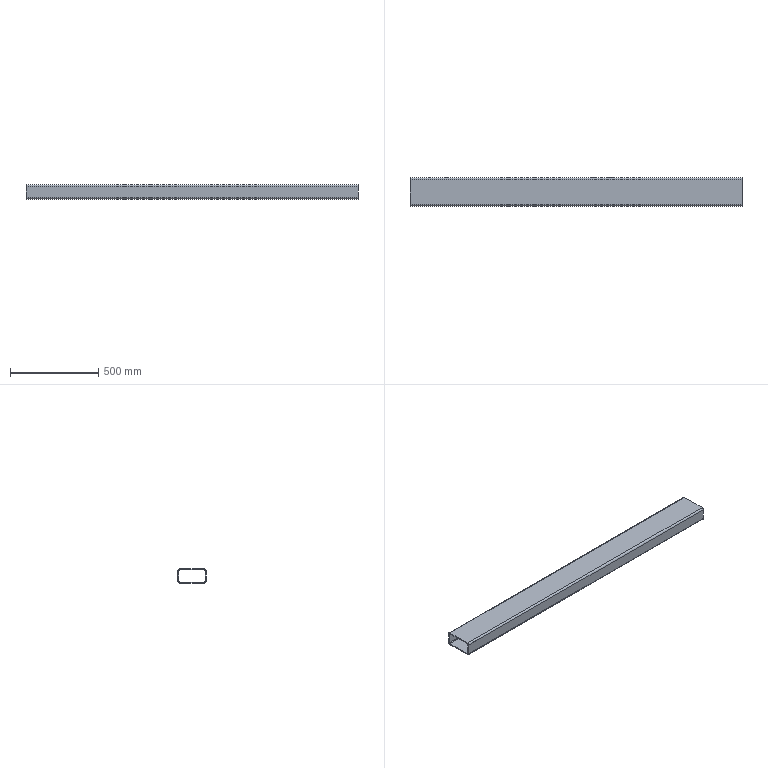Part | SolidWorks | features BaseBody 1 | 1 solid | 26 faces | box 1880 x 160 x 80 mm | volume 4199886 mm3 | cylinder 16 | plane 10 | commonest cylinder face diameters 14 x8 10 x4 20 x4
STEP:
#1=CARTESIAN_POINT('',(-837.,75.,-10.));
#2=VERTEX_POINT('',#1);
#3=CARTESIAN_POINT('',(-823.,75.,-10.));
#4=VERTEX_POINT('',#3);
#5=CARTESIAN_POINT('',(-830.,75.,-10.));
#6=DIRECTION('',(0.,-1.,0.));
#7=DIRECTION('',(0.,0.,-1.));
#8=AXIS2_PLACEMENT_3D('',#5,#6,#7);
#9=CIRCLE('',#8,7.);
#10=EDGE_CURVE('',#2,#4,#9,.T.);
#11=ORIENTED_EDGE('',*,*,#10,.T.);
#12=CARTESIAN_POINT('',(-823.,80.,-10.));
#13=VERTEX_POINT('',#12);
#14=CARTESIAN_POINT('',(-823.,100.,-10.));
#15=DIRECTION('',(0.,1.,0.));
#16=VECTOR('',#15,1000.);
#17=LINE('',#14,#16);
#18=EDGE_CURVE('',#4,#13,#17,.T.);
#19=ORIENTED_EDGE('',*,*,#18,.T.);
#20=CARTESIAN_POINT('',(-837.,80.,-10.));
#21=VERTEX_POINT('',#20);
#22=CARTESIAN_POINT('',(-830.,80.,-10.));
#23=DIRECTION('',(0.,-1.,0.));
#24=DIRECTION('',(0.,0.,-1.));
#25=AXIS2_PLACEMENT_3D('',#22,#23,#24);
#26=CIRCLE('',#25,7.);
#27=EDGE_CURVE('',#21,#13,#26,.T.);
#28=ORIENTED_EDGE('',*,*,#27,.F.);
#29=CARTESIAN_POINT('',(-837.,100.,-10.));
#30=DIRECTION('',(0.,1.,0.));
#31=VECTOR('',#30,1000.);
#32=LINE('',#29,#31);
#33=EDGE_CURVE('',#2,#21,#32,.T.);
#34=ORIENTED_EDGE('',*,*,#33,.F.);
#35=EDGE_LOOP('',(#11,#19,#28,#34));
#36=FACE_OUTER_BOUND('',#35,.T.);
#37=CARTESIAN_POINT('',(-830.,100.,-10.));
#38=DIRECTION('',(0.,1.,0.));
#39=DIRECTION('',(-1.,0.,0.));
#40=AXIS2_PLACEMENT_3D('',#37,#38,#39);
#41=CYLINDRICAL_SURFACE('',#40,7.);
#42=ADVANCED_FACE('',(#36),#41,.F.);
#43=CARTESIAN_POINT('',(-737.,75.,-10.));
#44=VERTEX_POINT('',#43);
#45=CARTESIAN_POINT('',(-723.,75.,-10.));
#46=VERTEX_POINT('',#45);
#47=CARTESIAN_POINT('',(-730.,75.,-10.));
#48=DIRECTION('',(0.,-1.,0.));
#49=DIRECTION('',(0.,0.,-1.));
#50=AXIS2_PLACEMENT_3D('',#47,#48,#49);
#51=CIRCLE('',#50,7.);
#52=EDGE_CURVE('',#44,#46,#51,.T.);
#53=ORIENTED_EDGE('',*,*,#52,.T.);
#54=CARTESIAN_POINT('',(-723.,80.,-10.));
#55=VERTEX_POINT('',#54);
#56=CARTESIAN_POINT('',(-723.,100.,-10.));
#57=DIRECTION('',(0.,1.,0.));
#58=VECTOR('',#57,1000.);
#59=LINE('',#56,#58);
#60=EDGE_CURVE('',#46,#55,#59,.T.);
#61=ORIENTED_EDGE('',*,*,#60,.T.);
#62=CARTESIAN_POINT('',(-737.,80.,-10.));
#63=VERTEX_POINT('',#62);
#64=CARTESIAN_POINT('',(-730.,80.,-10.));
#65=DIRECTION('',(0.,-1.,0.));
#66=DIRECTION('',(0.,0.,-1.));
#67=AXIS2_PLACEMENT_3D('',#64,#65,#66);
#68=CIRCLE('',#67,7.);
#69=EDGE_CURVE('',#63,#55,#68,.T.);
#70=ORIENTED_EDGE('',*,*,#69,.F.);
#71=CARTESIAN_POINT('',(-737.,100.,-10.));
#72=DIRECTION('',(0.,1.,0.));
#73=VECTOR('',#72,1000.);
#74=LINE('',#71,#73);
#75=EDGE_CURVE('',#44,#63,#74,.T.);
#76=ORIENTED_EDGE('',*,*,#75,.F.);
#77=EDGE_LOOP('',(#53,#61,#70,#76));
#78=FACE_OUTER_BOUND('',#77,.T.);
#79=CARTESIAN_POINT('',(-730.,100.,-10.));
#80=DIRECTION('',(0.,1.,0.));
#81=DIRECTION('',(-1.,0.,0.));
#82=AXIS2_PLACEMENT_3D('',#79,#80,#81);
#83=CYLINDRICAL_SURFACE('',#82,7.);
#84=ADVANCED_FACE('',(#78),#83,.F.);
#85=CARTESIAN_POINT('',(88.,75.,-10.));
#86=VERTEX_POINT('',#85);
#87=CARTESIAN_POINT('',(102.,75.,-10.));
#88=VERTEX_POINT('',#87);
#89=CARTESIAN_POINT('',(95.,75.,-10.));
#90=DIRECTION('',(0.,-1.,0.));
#91=DIRECTION('',(0.,0.,-1.));
#92=AXIS2_PLACEMENT_3D('',#89,#90,#91);
#93=CIRCLE('',#92,7.);
#94=EDGE_CURVE('',#86,#88,#93,.T.);
#95=ORIENTED_EDGE('',*,*,#94,.T.);
#96=CARTESIAN_POINT('',(102.,80.,-10.));
#97=VERTEX_POINT('',#96);
#98=CARTESIAN_POINT('',(102.,100.,-10.));
#99=DIRECTION('',(0.,1.,0.));
#100=VECTOR('',#99,1000.);
#101=LINE('',#98,#100);
#102=EDGE_CURVE('',#88,#97,#101,.T.);
#103=ORIENTED_EDGE('',*,*,#102,.T.);
#104=CARTESIAN_POINT('',(88.,80.,-10.));
#105=VERTEX_POINT('',#104);
#106=CARTESIAN_POINT('',(95.,80.,-10.));
#107=DIRECTION('',(0.,-1.,0.));
#108=DIRECTION('',(0.,0.,-1.));
#109=AXIS2_PLACEMENT_3D('',#106,#107,#108);
#110=CIRCLE('',#109,7.);
#111=EDGE_CURVE('',#105,#97,#110,.T.);
#112=ORIENTED_EDGE('',*,*,#111,.F.);
#113=CARTESIAN_POINT('',(88.,100.,-10.));
#114=DIRECTION('',(0.,1.,0.));
#115=VECTOR('',#114,1000.);
#116=LINE('',#113,#115);
#117=EDGE_CURVE('',#86,#105,#116,.T.);
#118=ORIENTED_EDGE('',*,*,#117,.F.);
#119=EDGE_LOOP('',(#95,#103,#112,#118));
#120=FACE_OUTER_BOUND('',#119,.T.);
#121=CARTESIAN_POINT('',(95.,100.,-10.));
#122=DIRECTION('',(0.,1.,0.));
#123=DIRECTION('',(-1.,0.,0.));
#124=AXIS2_PLACEMENT_3D('',#121,#122,#123);
#125=CYLINDRICAL_SURFACE('',#124,7.);
#126=ADVANCED_FACE('',(#120),#125,.F.);
#127=CARTESIAN_POINT('',(188.,75.,-10.));
#128=VERTEX_POINT('',#127);
#129=CARTESIAN_POINT('',(202.,75.,-10.));
#130=VERTEX_POINT('',#129);
#131=CARTESIAN_POINT('',(195.,75.,-10.));
#132=DIRECTION('',(0.,-1.,0.));
#133=DIRECTION('',(0.,0.,-1.));
#134=AXIS2_PLACEMENT_3D('',#131,#132,#133);
#135=CIRCLE('',#134,7.);
#136=EDGE_CURVE('',#128,#130,#135,.T.);
#137=ORIENTED_EDGE('',*,*,#136,.T.);
#138=CARTESIAN_POINT('',(202.,80.,-10.));
#139=VERTEX_POINT('',#138);
#140=CARTESIAN_POINT('',(202.,100.,-10.));
#141=DIRECTION('',(0.,1.,0.));
#142=VECTOR('',#141,1000.);
#143=LINE('',#140,#142);
#144=EDGE_CURVE('',#130,#139,#143,.T.);
#145=ORIENTED_EDGE('',*,*,#144,.T.);
#146=CARTESIAN_POINT('',(188.,80.,-10.));
#147=VERTEX_POINT('',#146);
#148=CARTESIAN_POINT('',(195.,80.,-10.));
#149=DIRECTION('',(0.,-1.,0.));
#150=DIRECTION('',(0.,0.,-1.));
#151=AXIS2_PLACEMENT_3D('',#148,#149,#150);
#152=CIRCLE('',#151,7.);
#153=EDGE_CURVE('',#147,#139,#152,.T.);
#154=ORIENTED_EDGE('',*,*,#153,.F.);
#155=CARTESIAN_POINT('',(188.,100.,-10.));
#156=DIRECTION('',(0.,1.,0.));
#157=VECTOR('',#156,1000.);
#158=LINE('',#155,#157);
#159=EDGE_CURVE('',#128,#147,#158,.T.);
#160=ORIENTED_EDGE('',*,*,#159,.F.);
#161=EDGE_LOOP('',(#137,#145,#154,#160));
#162=FACE_OUTER_BOUND('',#161,.T.);
#163=CARTESIAN_POINT('',(195.,100.,-10.));
#164=DIRECTION('',(0.,1.,0.));
#165=DIRECTION('',(-1.,0.,0.));
#166=AXIS2_PLACEMENT_3D('',#163,#164,#165);
#167=CYLINDRICAL_SURFACE('',#166,7.);
#168=ADVANCED_FACE('',(#162),#167,.F.);
#169=CARTESIAN_POINT('',(-940.,70.,-40.));
#170=VERTEX_POINT('',#169);
#171=CARTESIAN_POINT('',(-940.,80.,-30.));
#172=VERTEX_POINT('',#171);
#173=CARTESIAN_POINT('',(-940.,70.,-30.));
#174=DIRECTION('',(1.,0.,0.));
#175=DIRECTION('',(0.,0.,-1.));
#176=AXIS2_PLACEMENT_3D('',#173,#174,#175);
#177=CIRCLE('',#176,10.);
#178=EDGE_CURVE('',#170,#172,#177,.T.);
#179=ORIENTED_EDGE('',*,*,#178,.T.);
#180=CARTESIAN_POINT('',(940.,80.,-30.));
#181=VERTEX_POINT('',#180);
#182=CARTESIAN_POINT('',(940.,80.,-30.));
#183=DIRECTION('',(-1.,0.,0.));
#184=VECTOR('',#183,1000.);
#185=LINE('',#182,#184);
#186=EDGE_CURVE('',#181,#172,#185,.T.);
#187=ORIENTED_EDGE('',*,*,#186,.F.);
#188=CARTESIAN_POINT('',(940.,70.,-40.));
#189=VERTEX_POINT('',#188);
#190=CARTESIAN_POINT('',(940.,70.,-30.));
#191=DIRECTION('',(1.,0.,0.));
#192=DIRECTION('',(0.,0.,-1.));
#193=AXIS2_PLACEMENT_3D('',#190,#191,#192);
#194=CIRCLE('',#193,10.);
#195=EDGE_CURVE('',#189,#181,#194,.T.);
#196=ORIENTED_EDGE('',*,*,#195,.F.);
#197=CARTESIAN_POINT('',(940.,70.,-40.));
#198=DIRECTION('',(-1.,0.,0.));
#199=VECTOR('',#198,1000.);
#200=LINE('',#197,#199);
#201=EDGE_CURVE('',#189,#170,#200,.T.);
#202=ORIENTED_EDGE('',*,*,#201,.T.);
#203=EDGE_LOOP('',(#179,#187,#196,#202));
#204=FACE_OUTER_BOUND('',#203,.T.);
#205=CARTESIAN_POINT('',(940.,70.,-30.));
#206=DIRECTION('',(-1.,0.,0.));
#207=DIRECTION('',(0.,0.,1.));
#208=AXIS2_PLACEMENT_3D('',#205,#206,#207);
#209=CYLINDRICAL_SURFACE('',#208,10.);
#210=ADVANCED_FACE('',(#204),#209,.T.);
#211=ORIENTED_EDGE('',*,*,#27,.T.);
#212=CARTESIAN_POINT('',(-830.,80.,-10.));
#213=DIRECTION('',(0.,-1.,0.));
#214=DIRECTION('',(0.,0.,-1.));
#215=AXIS2_PLACEMENT_3D('',#212,#213,#214);
#216=CIRCLE('',#215,7.);
#217=EDGE_CURVE('',#13,#21,#216,.T.);
#218=ORIENTED_EDGE('',*,*,#217,.T.);
#219=EDGE_LOOP('',(#211,#218));
#220=FACE_BOUND('',#219,.T.);
#221=ORIENTED_EDGE('',*,*,#69,.T.);
#222=CARTESIAN_POINT('',(-730.,80.,-10.));
#223=DIRECTION('',(0.,-1.,0.));
#224=DIRECTION('',(0.,0.,-1.));
#225=AXIS2_PLACEMENT_3D('',#222,#223,#224);
#226=CIRCLE('',#225,7.);
#227=EDGE_CURVE('',#55,#63,#226,.T.);
#228=ORIENTED_EDGE('',*,*,#227,.T.);
#229=EDGE_LOOP('',(#221,#228));
#230=FACE_BOUND('',#229,.T.);
#231=ORIENTED_EDGE('',*,*,#111,.T.);
#232=CARTESIAN_POINT('',(95.,80.,-10.));
#233=DIRECTION('',(0.,-1.,0.));
#234=DIRECTION('',(0.,0.,-1.));
#235=AXIS2_PLACEMENT_3D('',#232,#233,#234);
#236=CIRCLE('',#235,7.);
#237=EDGE_CURVE('',#97,#105,#236,.T.);
#238=ORIENTED_EDGE('',*,*,#237,.T.);
#239=EDGE_LOOP('',(#231,#238));
#240=FACE_BOUND('',#239,.T.);
#241=ORIENTED_EDGE('',*,*,#153,.T.);
#242=CARTESIAN_POINT('',(195.,80.,-10.));
#243=DIRECTION('',(0.,-1.,0.));
#244=DIRECTION('',(0.,0.,-1.));
#245=AXIS2_PLACEMENT_3D('',#242,#243,#244);
#246=CIRCLE('',#245,7.);
#247=EDGE_CURVE('',#139,#147,#246,.T.);
#248=ORIENTED_EDGE('',*,*,#247,.T.);
#249=EDGE_LOOP('',(#241,#248));
#250=FACE_BOUND('',#249,.T.);
#251=CARTESIAN_POINT('',(-940.,80.,30.));
#252=VERTEX_POINT('',#251);
#253=CARTESIAN_POINT('',(-940.,80.,-30.));
#254=DIRECTION('',(0.,0.,1.));
#255=VECTOR('',#254,1000.);
#256=LINE('',#253,#255);
#257=EDGE_CURVE('',#172,#252,#256,.T.);
#258=ORIENTED_EDGE('',*,*,#257,.T.);
#259=CARTESIAN_POINT('',(940.,80.,30.));
#260=VERTEX_POINT('',#259);
#261=CARTESIAN_POINT('',(940.,80.,30.));
#262=DIRECTION('',(-1.,0.,0.));
#263=VECTOR('',#262,1000.);
#264=LINE('',#261,#263);
#265=EDGE_CURVE('',#260,#252,#264,.T.);
#266=ORIENTED_EDGE('',*,*,#265,.F.);
#267=CARTESIAN_POINT('',(940.,80.,-30.));
#268=DIRECTION('',(0.,0.,1.));
#269=VECTOR('',#268,1000.);
#270=LINE('',#267,#269);
#271=EDGE_CURVE('',#181,#260,#270,.T.);
#272=ORIENTED_EDGE('',*,*,#271,.F.);
#273=ORIENTED_EDGE('',*,*,#186,.T.);
#274=EDGE_LOOP('',(#258,#266,#272,#273));
#275=FACE_OUTER_BOUND('',#274,.T.);
#276=CARTESIAN_POINT('',(940.,80.,-30.));
#277=DIRECTION('',(0.,-1.,0.));
#278=DIRECTION('',(0.,0.,-1.));
#279=AXIS2_PLACEMENT_3D('',#276,#277,#278);
#280=PLANE('',#279);
#281=ADVANCED_FACE('',(#220,#230,#240,#250,#275),#280,.F.);
#282=CARTESIAN_POINT('',(-940.,70.,40.));
#283=VERTEX_POINT('',#282);
#284=CARTESIAN_POINT('',(-940.,70.,30.));
#285=DIRECTION('',(1.,0.,0.));
#286=DIRECTION('',(0.,0.,-1.));
#287=AXIS2_PLACEMENT_3D('',#284,#285,#286);
#288=CIRCLE('',#287,10.);
#289=EDGE_CURVE('',#252,#283,#288,.T.);
#290=ORIENTED_EDGE('',*,*,#289,.T.);
#291=CARTESIAN_POINT('',(940.,70.,40.));
#292=VERTEX_POINT('',#291);
#293=CARTESIAN_POINT('',(940.,70.,40.));
#294=DIRECTION('',(-1.,0.,0.));
#295=VECTOR('',#294,1000.);
#296=LINE('',#293,#295);
#297=EDGE_CURVE('',#292,#283,#296,.T.);
#298=ORIENTED_EDGE('',*,*,#297,.F.);
#299=CARTESIAN_POINT('',(940.,70.,30.));
#300=DIRECTION('',(1.,0.,0.));
#301=DIRECTION('',(0.,0.,-1.));
#302=AXIS2_PLACEMENT_3D('',#299,#300,#301);
#303=CIRCLE('',#302,10.);
#304=EDGE_CURVE('',#260,#292,#303,.T.);
#305=ORIENTED_EDGE('',*,*,#304,.F.);
#306=ORIENTED_EDGE('',*,*,#265,.T.);
#307=EDGE_LOOP('',(#290,#298,#305,#306));
#308=FACE_OUTER_BOUND('',#307,.T.);
#309=CARTESIAN_POINT('',(940.,70.,30.));
#310=DIRECTION('',(-1.,0.,0.));
#311=DIRECTION('',(0.,0.,1.));
#312=AXIS2_PLACEMENT_3D('',#309,#310,#311);
#313=CYLINDRICAL_SURFACE('',#312,10.);
#314=ADVANCED_FACE('',(#308),#313,.T.);
#315=CARTESIAN_POINT('',(-940.,-70.,40.));
#316=VERTEX_POINT('',#315);
#317=CARTESIAN_POINT('',(-940.,-70.,40.));
#318=DIRECTION('',(0.,-1.,0.));
#319=VECTOR('',#318,1000.);
#320=LINE('',#317,#319);
#321=EDGE_CURVE('',#283,#316,#320,.T.);
#322=ORIENTED_EDGE('',*,*,#321,.T.);
#323=CARTESIAN_POINT('',(940.,-70.,40.));
#324=VERTEX_POINT('',#323);
#325=CARTESIAN_POINT('',(940.,-70.,40.));
#326=DIRECTION('',(-1.,0.,0.));
#327=VECTOR('',#326,1000.);
#328=LINE('',#325,#327);
#329=EDGE_CURVE('',#324,#316,#328,.T.);
#330=ORIENTED_EDGE('',*,*,#329,.F.);
#331=CARTESIAN_POINT('',(940.,-70.,40.));
#332=DIRECTION('',(0.,-1.,0.));
#333=VECTOR('',#332,1000.);
#334=LINE('',#331,#333);
#335=EDGE_CURVE('',#292,#324,#334,.T.);
#336=ORIENTED_EDGE('',*,*,#335,.F.);
#337=ORIENTED_EDGE('',*,*,#297,.T.);
#338=EDGE_LOOP('',(#322,#330,#336,#337));
#339=FACE_OUTER_BOUND('',#338,.T.);
#340=CARTESIAN_POINT('',(940.,-70.,40.));
#341=DIRECTION('',(0.,0.,-1.));
#342=DIRECTION('',(0.,1.,0.));
#343=AXIS2_PLACEMENT_3D('',#340,#341,#342);
#344=PLANE('',#343);
#345=ADVANCED_FACE('',(#339),#344,.F.);
#346=CARTESIAN_POINT('',(-940.,-80.,30.));
#347=VERTEX_POINT('',#346);
#348=CARTESIAN_POINT('',(-940.,-70.,30.));
#349=DIRECTION('',(1.,0.,0.));
#350=DIRECTION('',(0.,0.,-1.));
#351=AXIS2_PLACEMENT_3D('',#348,#349,#350);
#352=CIRCLE('',#351,10.);
#353=EDGE_CURVE('',#316,#347,#352,.T.);
#354=ORIENTED_EDGE('',*,*,#353,.T.);
#355=CARTESIAN_POINT('',(940.,-80.,30.));
#356=VERTEX_POINT('',#355);
#357=CARTESIAN_POINT('',(940.,-80.,30.));
#358=DIRECTION('',(-1.,0.,0.));
#359=VECTOR('',#358,1000.);
#360=LINE('',#357,#359);
#361=EDGE_CURVE('',#356,#347,#360,.T.);
#362=ORIENTED_EDGE('',*,*,#361,.F.);
#363=CARTESIAN_POINT('',(940.,-70.,30.));
#364=DIRECTION('',(1.,0.,0.));
#365=DIRECTION('',(0.,0.,-1.));
#366=AXIS2_PLACEMENT_3D('',#363,#364,#365);
#367=CIRCLE('',#366,10.);
#368=EDGE_CURVE('',#324,#356,#367,.T.);
#369=ORIENTED_EDGE('',*,*,#368,.F.);
#370=ORIENTED_EDGE('',*,*,#329,.T.);
#371=EDGE_LOOP('',(#354,#362,#369,#370));
#372=FACE_OUTER_BOUND('',#371,.T.);
#373=CARTESIAN_POINT('',(940.,-70.,30.));
#374=DIRECTION('',(-1.,0.,0.));
#375=DIRECTION('',(0.,0.,1.));
#376=AXIS2_PLACEMENT_3D('',#373,#374,#375);
#377=CYLINDRICAL_SURFACE('',#376,10.);
#378=ADVANCED_FACE('',(#372),#377,.T.);
#379=CARTESIAN_POINT('',(-940.,-80.,-30.));
#380=VERTEX_POINT('',#379);
#381=CARTESIAN_POINT('',(-940.,-80.,30.));
#382=DIRECTION('',(0.,0.,-1.));
#383=VECTOR('',#382,1000.);
#384=LINE('',#381,#383);
#385=EDGE_CURVE('',#347,#380,#384,.T.);
#386=ORIENTED_EDGE('',*,*,#385,.T.);
#387=CARTESIAN_POINT('',(940.,-80.,-30.));
#388=VERTEX_POINT('',#387);
#389=CARTESIAN_POINT('',(940.,-80.,-30.));
#390=DIRECTION('',(-1.,0.,0.));
#391=VECTOR('',#390,1000.);
#392=LINE('',#389,#391);
#393=EDGE_CURVE('',#388,#380,#392,.T.);
#394=ORIENTED_EDGE('',*,*,#393,.F.);
#395=CARTESIAN_POINT('',(940.,-80.,30.));
#396=DIRECTION('',(0.,0.,-1.));
#397=VECTOR('',#396,1000.);
#398=LINE('',#395,#397);
#399=EDGE_CURVE('',#356,#388,#398,.T.);
#400=ORIENTED_EDGE('',*,*,#399,.F.);
#401=ORIENTED_EDGE('',*,*,#361,.T.);
#402=EDGE_LOOP('',(#386,#394,#400,#401));
#403=FACE_OUTER_BOUND('',#402,.T.);
#404=CARTESIAN_POINT('',(940.,-80.,30.));
#405=DIRECTION('',(0.,1.,0.));
#406=DIRECTION('',(0.,0.,1.));
#407=AXIS2_PLACEMENT_3D('',#404,#405,#406);
#408=PLANE('',#407);
#409=ADVANCED_FACE('',(#403),#408,.F.);
#410=CARTESIAN_POINT('',(-940.,-70.,-40.));
#411=VERTEX_POINT('',#410);
#412=CARTESIAN_POINT('',(-940.,-70.,-30.));
#413=DIRECTION('',(1.,0.,0.));
#414=DIRECTION('',(0.,0.,-1.));
#415=AXIS2_PLACEMENT_3D('',#412,#413,#414);
#416=CIRCLE('',#415,10.);
#417=EDGE_CURVE('',#380,#411,#416,.T.);
#418=ORIENTED_EDGE('',*,*,#417,.T.);
#419=CARTESIAN_POINT('',(940.,-70.,-40.));
#420=VERTEX_POINT('',#419);
#421=CARTESIAN_POINT('',(940.,-70.,-40.));
#422=DIRECTION('',(-1.,0.,0.));
#423=VECTOR('',#422,1000.);
#424=LINE('',#421,#423);
#425=EDGE_CURVE('',#420,#411,#424,.T.);
#426=ORIENTED_EDGE('',*,*,#425,.F.);
#427=CARTESIAN_POINT('',(940.,-70.,-30.));
#428=DIRECTION('',(1.,0.,0.));
#429=DIRECTION('',(0.,0.,-1.));
#430=AXIS2_PLACEMENT_3D('',#427,#428,#429);
#431=CIRCLE('',#430,10.);
#432=EDGE_CURVE('',#388,#420,#431,.T.);
#433=ORIENTED_EDGE('',*,*,#432,.F.);
#434=ORIENTED_EDGE('',*,*,#393,.T.);
#435=EDGE_LOOP('',(#418,#426,#433,#434));
#436=FACE_OUTER_BOUND('',#435,.T.);
#437=CARTESIAN_POINT('',(940.,-70.,-30.));
#438=DIRECTION('',(-1.,0.,0.));
#439=DIRECTION('',(0.,0.,1.));
#440=AXIS2_PLACEMENT_3D('',#437,#438,#439);
#441=CYLINDRICAL_SURFACE('',#440,10.);
#442=ADVANCED_FACE('',(#436),#441,.T.);
#443=CARTESIAN_POINT('',(-940.,75.,30.));
#444=VERTEX_POINT('',#443);
#445=CARTESIAN_POINT('',(-940.,70.,35.));
#446=VERTEX_POINT('',#445);
#447=CARTESIAN_POINT('',(-940.,70.,30.));
#448=DIRECTION('',(1.,0.,0.));
#449=DIRECTION('',(0.,0.,-1.));
#450=AXIS2_PLACEMENT_3D('',#447,#448,#449);
#451=CIRCLE('',#450,5.);
#452=EDGE_CURVE('',#444,#446,#451,.T.);
#453=ORIENTED_EDGE('',*,*,#452,.F.);
#454=CARTESIAN_POINT('',(940.,75.,30.));
#455=VERTEX_POINT('',#454);
#456=CARTESIAN_POINT('',(940.,75.,30.));
#457=DIRECTION('',(-1.,0.,0.));
#458=VECTOR('',#457,1000.);
#459=LINE('',#456,#458);
#460=EDGE_CURVE('',#455,#444,#459,.T.);
#461=ORIENTED_EDGE('',*,*,#460,.F.);
#462=CARTESIAN_POINT('',(940.,70.,35.));
#463=VERTEX_POINT('',#462);
#464=CARTESIAN_POINT('',(940.,70.,30.));
#465=DIRECTION('',(1.,0.,0.));
#466=DIRECTION('',(0.,0.,-1.));
#467=AXIS2_PLACEMENT_3D('',#464,#465,#466);
#468=CIRCLE('',#467,5.);
#469=EDGE_CURVE('',#455,#463,#468,.T.);
#470=ORIENTED_EDGE('',*,*,#469,.T.);
#471=CARTESIAN_POINT('',(940.,70.,35.));
#472=DIRECTION('',(-1.,0.,0.));
#473=VECTOR('',#472,1000.);
#474=LINE('',#471,#473);
#475=EDGE_CURVE('',#463,#446,#474,.T.);
#476=ORIENTED_EDGE('',*,*,#475,.T.);
#477=EDGE_LOOP('',(#453,#461,#470,#476));
#478=FACE_OUTER_BOUND('',#477,.T.);
#479=CARTESIAN_POINT('',(940.,70.,30.));
#480=DIRECTION('',(-1.,0.,0.));
#481=DIRECTION('',(0.,0.,1.));
#482=AXIS2_PLACEMENT_3D('',#479,#480,#481);
#483=CYLINDRICAL_SURFACE('',#482,5.);
#484=ADVANCED_FACE('',(#478),#483,.F.);
#485=ORIENTED_EDGE('',*,*,#10,.F.);
#486=CARTESIAN_POINT('',(-830.,75.,-10.));
#487=DIRECTION('',(0.,-1.,0.));
#488=DIRECTION('',(0.,0.,-1.));
#489=AXIS2_PLACEMENT_3D('',#486,#487,#488);
#490=CIRCLE('',#489,7.);
#491=EDGE_CURVE('',#4,#2,#490,.T.);
#492=ORIENTED_EDGE('',*,*,#491,.F.);
#493=EDGE_LOOP('',(#485,#492));
#494=FACE_BOUND('',#493,.T.);
#495=ORIENTED_EDGE('',*,*,#52,.F.);
#496=CARTESIAN_POINT('',(-730.,75.,-10.));
#497=DIRECTION('',(0.,-1.,0.));
#498=DIRECTION('',(0.,0.,-1.));
#499=AXIS2_PLACEMENT_3D('',#496,#497,#498);
#500=CIRCLE('',#499,7.);
#501=EDGE_CURVE('',#46,#44,#500,.T.);
#502=ORIENTED_EDGE('',*,*,#501,.F.);
#503=EDGE_LOOP('',(#495,#502));
#504=FACE_BOUND('',#503,.T.);
#505=ORIENTED_EDGE('',*,*,#94,.F.);
#506=CARTESIAN_POINT('',(95.,75.,-10.));
#507=DIRECTION('',(0.,-1.,0.));
#508=DIRECTION('',(0.,0.,-1.));
#509=AXIS2_PLACEMENT_3D('',#506,#507,#508);
#510=CIRCLE('',#509,7.);
#511=EDGE_CURVE('',#88,#86,#510,.T.);
#512=ORIENTED_EDGE('',*,*,#511,.F.);
#513=EDGE_LOOP('',(#505,#512));
#514=FACE_BOUND('',#513,.T.);
#515=ORIENTED_EDGE('',*,*,#136,.F.);
#516=CARTESIAN_POINT('',(195.,75.,-10.));
#517=DIRECTION('',(0.,-1.,0.));
#518=DIRECTION('',(0.,0.,-1.));
#519=AXIS2_PLACEMENT_3D('',#516,#517,#518);
#520=CIRCLE('',#519,7.);
#521=EDGE_CURVE('',#130,#128,#520,.T.);
#522=ORIENTED_EDGE('',*,*,#521,.F.);
#523=EDGE_LOOP('',(#515,#522));
#524=FACE_BOUND('',#523,.T.);
#525=CARTESIAN_POINT('',(-940.,75.,-30.));
#526=VERTEX_POINT('',#525);
#527=CARTESIAN_POINT('',(-940.,75.,-30.));
#528=DIRECTION('',(0.,0.,1.));
#529=VECTOR('',#528,1000.);
#530=LINE('',#527,#529);
#531=EDGE_CURVE('',#526,#444,#530,.T.);
#532=ORIENTED_EDGE('',*,*,#531,.F.);
#533=CARTESIAN_POINT('',(940.,75.,-30.));
#534=VERTEX_POINT('',#533);
#535=CARTESIAN_POINT('',(940.,75.,-30.));
#536=DIRECTION('',(-1.,0.,0.));
#537=VECTOR('',#536,1000.);
#538=LINE('',#535,#537);
#539=EDGE_CURVE('',#534,#526,#538,.T.);
#540=ORIENTED_EDGE('',*,*,#539,.F.);
#541=CARTESIAN_POINT('',(940.,75.,-30.));
#542=DIRECTION('',(0.,0.,1.));
#543=VECTOR('',#542,1000.);
#544=LINE('',#541,#543);
#545=EDGE_CURVE('',#534,#455,#544,.T.);
#546=ORIENTED_EDGE('',*,*,#545,.T.);
#547=ORIENTED_EDGE('',*,*,#460,.T.);
#548=EDGE_LOOP('',(#532,#540,#546,#547));
#549=FACE_OUTER_BOUND('',#548,.T.);
#550=CARTESIAN_POINT('',(940.,75.,-30.));
#551=DIRECTION('',(0.,-1.,0.));
#552=DIRECTION('',(0.,0.,-1.));
#553=AXIS2_PLACEMENT_3D('',#550,#551,#552);
#554=PLANE('',#553);
#555=ADVANCED_FACE('',(#494,#504,#514,#524,#549),#554,.T.);
#556=CARTESIAN_POINT('',(-940.,70.,-35.));
#557=VERTEX_POINT('',#556);
#558=CARTESIAN_POINT('',(-940.,70.,-30.));
#559=DIRECTION('',(1.,0.,0.));
#560=DIRECTION('',(0.,0.,-1.));
#561=AXIS2_PLACEMENT_3D('',#558,#559,#560);
#562=CIRCLE('',#561,5.);
#563=EDGE_CURVE('',#557,#526,#562,.T.);
#564=ORIENTED_EDGE('',*,*,#563,.F.);
#565=CARTESIAN_POINT('',(940.,70.,-35.));
#566=VERTEX_POINT('',#565);
#567=CARTESIAN_POINT('',(940.,70.,-35.));
#568=DIRECTION('',(-1.,0.,0.));
#569=VECTOR('',#568,1000.);
#570=LINE('',#567,#569);
#571=EDGE_CURVE('',#566,#557,#570,.T.);
#572=ORIENTED_EDGE('',*,*,#571,.F.);
#573=CARTESIAN_POINT('',(940.,70.,-30.));
#574=DIRECTION('',(1.,0.,0.));
#575=DIRECTION('',(0.,0.,-1.));
#576=AXIS2_PLACEMENT_3D('',#573,#574,#575);
#577=CIRCLE('',#576,5.);
#578=EDGE_CURVE('',#566,#534,#577,.T.);
#579=ORIENTED_EDGE('',*,*,#578,.T.);
#580=ORIENTED_EDGE('',*,*,#539,.T.);
#581=EDGE_LOOP('',(#564,#572,#579,#580));
#582=FACE_OUTER_BOUND('',#581,.T.);
#583=CARTESIAN_POINT('',(940.,70.,-30.));
#584=DIRECTION('',(-1.,0.,0.));
#585=DIRECTION('',(0.,0.,1.));
#586=AXIS2_PLACEMENT_3D('',#583,#584,#585);
#587=CYLINDRICAL_SURFACE('',#586,5.);
#588=ADVANCED_FACE('',(#582),#587,.F.);
#589=CARTESIAN_POINT('',(-940.,-70.,-35.));
#590=VERTEX_POINT('',#589);
#591=CARTESIAN_POINT('',(-940.,70.,-35.));
#592=DIRECTION('',(0.,1.,0.));
#593=VECTOR('',#592,1000.);
#594=LINE('',#591,#593);
#595=EDGE_CURVE('',#590,#557,#594,.T.);
#596=ORIENTED_EDGE('',*,*,#595,.F.);
#597=CARTESIAN_POINT('',(940.,-70.,-35.));
#598=VERTEX_POINT('',#597);
#599=CARTESIAN_POINT('',(940.,-70.,-35.));
#600=DIRECTION('',(-1.,0.,0.));
#601=VECTOR('',#600,1000.);
#602=LINE('',#599,#601);
#603=EDGE_CURVE('',#598,#590,#602,.T.);
#604=ORIENTED_EDGE('',*,*,#603,.F.);
#605=CARTESIAN_POINT('',(940.,70.,-35.));
#606=DIRECTION('',(0.,1.,0.));
#607=VECTOR('',#606,1000.);
#608=LINE('',#605,#607);
#609=EDGE_CURVE('',#598,#566,#608,.T.);
#610=ORIENTED_EDGE('',*,*,#609,.T.);
#611=ORIENTED_EDGE('',*,*,#571,.T.);
#612=EDGE_LOOP('',(#596,#604,#610,#611));
#613=FACE_OUTER_BOUND('',#612,.T.);
#614=CARTESIAN_POINT('',(940.,70.,-35.));
#615=DIRECTION('',(0.,0.,1.));
#616=DIRECTION('',(1.,0.,0.));
#617=AXIS2_PLACEMENT_3D('',#614,#615,#616);
#618=PLANE('',#617);
#619=ADVANCED_FACE('',(#613),#618,.T.);
#620=CARTESIAN_POINT('',(-940.,-75.,-30.));
#621=VERTEX_POINT('',#620);
#622=CARTESIAN_POINT('',(-940.,-70.,-30.));
#623=DIRECTION('',(1.,0.,0.));
#624=DIRECTION('',(0.,0.,-1.));
#625=AXIS2_PLACEMENT_3D('',#622,#623,#624);
#626=CIRCLE('',#625,5.);
#627=EDGE_CURVE('',#621,#590,#626,.T.);
#628=ORIENTED_EDGE('',*,*,#627,.F.);
#629=CARTESIAN_POINT('',(940.,-75.,-30.));
#630=VERTEX_POINT('',#629);
#631=CARTESIAN_POINT('',(940.,-75.,-30.));
#632=DIRECTION('',(-1.,0.,0.));
#633=VECTOR('',#632,1000.);
#634=LINE('',#631,#633);
#635=EDGE_CURVE('',#630,#621,#634,.T.);
#636=ORIENTED_EDGE('',*,*,#635,.F.);
#637=CARTESIAN_POINT('',(940.,-70.,-30.));
#638=DIRECTION('',(1.,0.,0.));
#639=DIRECTION('',(0.,0.,-1.));
#640=AXIS2_PLACEMENT_3D('',#637,#638,#639);
#641=CIRCLE('',#640,5.);
#642=EDGE_CURVE('',#630,#598,#641,.T.);
#643=ORIENTED_EDGE('',*,*,#642,.T.);
#644=ORIENTED_EDGE('',*,*,#603,.T.);
#645=EDGE_LOOP('',(#628,#636,#643,#644));
#646=FACE_OUTER_BOUND('',#645,.T.);
#647=CARTESIAN_POINT('',(940.,-70.,-30.));
#648=DIRECTION('',(-1.,0.,0.));
#649=DIRECTION('',(0.,0.,1.));
#650=AXIS2_PLACEMENT_3D('',#647,#648,#649);
#651=CYLINDRICAL_SURFACE('',#650,5.);
#652=ADVANCED_FACE('',(#646),#651,.F.);
#653=CARTESIAN_POINT('',(-940.,-75.,30.));
#654=VERTEX_POINT('',#653);
#655=CARTESIAN_POINT('',(-940.,-75.,30.));
#656=DIRECTION('',(0.,0.,-1.));
#657=VECTOR('',#656,1000.);
#658=LINE('',#655,#657);
#659=EDGE_CURVE('',#654,#621,#658,.T.);
#660=ORIENTED_EDGE('',*,*,#659,.F.);
#661=CARTESIAN_POINT('',(940.,-75.,30.));
#662=VERTEX_POINT('',#661);
#663=CARTESIAN_POINT('',(940.,-75.,30.));
#664=DIRECTION('',(-1.,0.,0.));
#665=VECTOR('',#664,1000.);
#666=LINE('',#663,#665);
#667=EDGE_CURVE('',#662,#654,#666,.T.);
#668=ORIENTED_EDGE('',*,*,#667,.F.);
#669=CARTESIAN_POINT('',(940.,-75.,30.));
#670=DIRECTION('',(0.,0.,-1.));
#671=VECTOR('',#670,1000.);
#672=LINE('',#669,#671);
#673=EDGE_CURVE('',#662,#630,#672,.T.);
#674=ORIENTED_EDGE('',*,*,#673,.T.);
#675=ORIENTED_EDGE('',*,*,#635,.T.);
#676=EDGE_LOOP('',(#660,#668,#674,#675));
#677=FACE_OUTER_BOUND('',#676,.T.);
#678=CARTESIAN_POINT('',(940.,-75.,30.));
#679=DIRECTION('',(0.,1.,0.));
#680=DIRECTION('',(0.,0.,1.));
#681=AXIS2_PLACEMENT_3D('',#678,#679,#680);
#682=PLANE('',#681);
#683=ADVANCED_FACE('',(#677),#682,.T.);
#684=CARTESIAN_POINT('',(-940.,-70.,35.));
#685=VERTEX_POINT('',#684);
#686=CARTESIAN_POINT('',(-940.,-70.,30.));
#687=DIRECTION('',(1.,0.,0.));
#688=DIRECTION('',(0.,0.,-1.));
#689=AXIS2_PLACEMENT_3D('',#686,#687,#688);
#690=CIRCLE('',#689,5.);
#691=EDGE_CURVE('',#685,#654,#690,.T.);
#692=ORIENTED_EDGE('',*,*,#691,.F.);
#693=CARTESIAN_POINT('',(940.,-70.,35.));
#694=VERTEX_POINT('',#693);
#695=CARTESIAN_POINT('',(940.,-70.,35.));
#696=DIRECTION('',(-1.,0.,0.));
#697=VECTOR('',#696,1000.);
#698=LINE('',#695,#697);
#699=EDGE_CURVE('',#694,#685,#698,.T.);
#700=ORIENTED_EDGE('',*,*,#699,.F.);
#701=CARTESIAN_POINT('',(940.,-70.,30.));
#702=DIRECTION('',(1.,0.,0.));
#703=DIRECTION('',(0.,0.,-1.));
#704=AXIS2_PLACEMENT_3D('',#701,#702,#703);
#705=CIRCLE('',#704,5.);
#706=EDGE_CURVE('',#694,#662,#705,.T.);
#707=ORIENTED_EDGE('',*,*,#706,.T.);
#708=ORIENTED_EDGE('',*,*,#667,.T.);
#709=EDGE_LOOP('',(#692,#700,#707,#708));
#710=FACE_OUTER_BOUND('',#709,.T.);
#711=CARTESIAN_POINT('',(940.,-70.,30.));
#712=DIRECTION('',(-1.,0.,0.));
#713=DIRECTION('',(0.,0.,1.));
#714=AXIS2_PLACEMENT_3D('',#711,#712,#713);
#715=CYLINDRICAL_SURFACE('',#714,5.);
#716=ADVANCED_FACE('',(#710),#715,.F.);
#717=CARTESIAN_POINT('',(-940.,-70.,35.));
#718=DIRECTION('',(0.,-1.,0.));
#719=VECTOR('',#718,1000.);
#720=LINE('',#717,#719);
#721=EDGE_CURVE('',#446,#685,#720,.T.);
#722=ORIENTED_EDGE('',*,*,#721,.F.);
#723=ORIENTED_EDGE('',*,*,#475,.F.);
#724=CARTESIAN_POINT('',(940.,-70.,35.));
#725=DIRECTION('',(0.,-1.,0.));
#726=VECTOR('',#725,1000.);
#727=LINE('',#724,#726);
#728=EDGE_CURVE('',#463,#694,#727,.T.);
#729=ORIENTED_EDGE('',*,*,#728,.T.);
#730=ORIENTED_EDGE('',*,*,#699,.T.);
#731=EDGE_LOOP('',(#722,#723,#729,#730));
#732=FACE_OUTER_BOUND('',#731,.T.);
#733=CARTESIAN_POINT('',(940.,-70.,35.));
#734=DIRECTION('',(0.,0.,-1.));
#735=DIRECTION('',(0.,1.,0.));
#736=AXIS2_PLACEMENT_3D('',#733,#734,#735);
#737=PLANE('',#736);
#738=ADVANCED_FACE('',(#732),#737,.T.);
#739=CARTESIAN_POINT('',(-940.,70.,-40.));
#740=DIRECTION('',(0.,1.,0.));
#741=VECTOR('',#740,1000.);
#742=LINE('',#739,#741);
#743=EDGE_CURVE('',#411,#170,#742,.T.);
#744=ORIENTED_EDGE('',*,*,#743,.T.);
#745=ORIENTED_EDGE('',*,*,#201,.F.);
#746=CARTESIAN_POINT('',(940.,70.,-40.));
#747=DIRECTION('',(0.,1.,0.));
#748=VECTOR('',#747,1000.);
#749=LINE('',#746,#748);
#750=EDGE_CURVE('',#420,#189,#749,.T.);
#751=ORIENTED_EDGE('',*,*,#750,.F.);
#752=ORIENTED_EDGE('',*,*,#425,.T.);
#753=EDGE_LOOP('',(#744,#745,#751,#752));
#754=FACE_OUTER_BOUND('',#753,.T.);
#755=CARTESIAN_POINT('',(940.,70.,-40.));
#756=DIRECTION('',(0.,0.,1.));
#757=DIRECTION('',(1.,0.,0.));
#758=AXIS2_PLACEMENT_3D('',#755,#756,#757);
#759=PLANE('',#758);
#760=ADVANCED_FACE('',(#754),#759,.F.);
#761=ORIENTED_EDGE('',*,*,#469,.F.);
#762=ORIENTED_EDGE('',*,*,#545,.F.);
#763=ORIENTED_EDGE('',*,*,#578,.F.);
#764=ORIENTED_EDGE('',*,*,#609,.F.);
#765=ORIENTED_EDGE('',*,*,#642,.F.);
#766=ORIENTED_EDGE('',*,*,#673,.F.);
#767=ORIENTED_EDGE('',*,*,#706,.F.);
#768=ORIENTED_EDGE('',*,*,#728,.F.);
#769=EDGE_LOOP('',(#761,#762,#763,#764,#765,#766,#767,#768));
#770=FACE_BOUND('',#769,.T.);
#771=ORIENTED_EDGE('',*,*,#195,.T.);
#772=ORIENTED_EDGE('',*,*,#271,.T.);
#773=ORIENTED_EDGE('',*,*,#304,.T.);
#774=ORIENTED_EDGE('',*,*,#335,.T.);
#775=ORIENTED_EDGE('',*,*,#368,.T.);
#776=ORIENTED_EDGE('',*,*,#399,.T.);
#777=ORIENTED_EDGE('',*,*,#432,.T.);
#778=ORIENTED_EDGE('',*,*,#750,.T.);
#779=EDGE_LOOP('',(#771,#772,#773,#774,#775,#776,#777,#778));
#780=FACE_OUTER_BOUND('',#779,.T.);
#781=CARTESIAN_POINT('',(940.,70.,-30.));
#782=DIRECTION('',(1.,0.,0.));
#783=DIRECTION('',(0.,0.,-1.));
#784=AXIS2_PLACEMENT_3D('',#781,#782,#783);
#785=PLANE('',#784);
#786=ADVANCED_FACE('',(#770,#780),#785,.T.);
#787=ORIENTED_EDGE('',*,*,#452,.T.);
#788=ORIENTED_EDGE('',*,*,#721,.T.);
#789=ORIENTED_EDGE('',*,*,#691,.T.);
#790=ORIENTED_EDGE('',*,*,#659,.T.);
#791=ORIENTED_EDGE('',*,*,#627,.T.);
#792=ORIENTED_EDGE('',*,*,#595,.T.);
#793=ORIENTED_EDGE('',*,*,#563,.T.);
#794=ORIENTED_EDGE('',*,*,#531,.T.);
#795=EDGE_LOOP('',(#787,#788,#789,#790,#791,#792,#793,#794));
#796=FACE_BOUND('',#795,.T.);
#797=ORIENTED_EDGE('',*,*,#178,.F.);
#798=ORIENTED_EDGE('',*,*,#743,.F.);
#799=ORIENTED_EDGE('',*,*,#417,.F.);
#800=ORIENTED_EDGE('',*,*,#385,.F.);
#801=ORIENTED_EDGE('',*,*,#353,.F.);
#802=ORIENTED_EDGE('',*,*,#321,.F.);
#803=ORIENTED_EDGE('',*,*,#289,.F.);
#804=ORIENTED_EDGE('',*,*,#257,.F.);
#805=EDGE_LOOP('',(#797,#798,#799,#800,#801,#802,#803,#804));
#806=FACE_OUTER_BOUND('',#805,.T.);
#807=CARTESIAN_POINT('',(-940.,70.,-30.));
#808=DIRECTION('',(1.,0.,0.));
#809=DIRECTION('',(0.,0.,-1.));
#810=AXIS2_PLACEMENT_3D('',#807,#808,#809);
#811=PLANE('',#810);
#812=ADVANCED_FACE('',(#796,#806),#811,.F.);
#813=ORIENTED_EDGE('',*,*,#144,.F.);
#814=ORIENTED_EDGE('',*,*,#521,.T.);
#815=ORIENTED_EDGE('',*,*,#159,.T.);
#816=ORIENTED_EDGE('',*,*,#247,.F.);
#817=EDGE_LOOP('',(#813,#814,#815,#816));
#818=FACE_OUTER_BOUND('',#817,.T.);
#819=CARTESIAN_POINT('',(195.,100.,-10.));
#820=DIRECTION('',(0.,1.,0.));
#821=DIRECTION('',(-1.,0.,0.));
#822=AXIS2_PLACEMENT_3D('',#819,#820,#821);
#823=CYLINDRICAL_SURFACE('',#822,7.);
#824=ADVANCED_FACE('',(#818),#823,.F.);
#825=ORIENTED_EDGE('',*,*,#102,.F.);
#826=ORIENTED_EDGE('',*,*,#511,.T.);
#827=ORIENTED_EDGE('',*,*,#117,.T.);
#828=ORIENTED_EDGE('',*,*,#237,.F.);
#829=EDGE_LOOP('',(#825,#826,#827,#828));
#830=FACE_OUTER_BOUND('',#829,.T.);
#831=CARTESIAN_POINT('',(95.,100.,-10.));
#832=DIRECTION('',(0.,1.,0.));
#833=DIRECTION('',(-1.,0.,0.));
#834=AXIS2_PLACEMENT_3D('',#831,#832,#833);
#835=CYLINDRICAL_SURFACE('',#834,7.);
#836=ADVANCED_FACE('',(#830),#835,.F.);
#837=ORIENTED_EDGE('',*,*,#60,.F.);
#838=ORIENTED_EDGE('',*,*,#501,.T.);
#839=ORIENTED_EDGE('',*,*,#75,.T.);
#840=ORIENTED_EDGE('',*,*,#227,.F.);
#841=EDGE_LOOP('',(#837,#838,#839,#840));
#842=FACE_OUTER_BOUND('',#841,.T.);
#843=CARTESIAN_POINT('',(-730.,100.,-10.));
#844=DIRECTION('',(0.,1.,0.));
#845=DIRECTION('',(-1.,0.,0.));
#846=AXIS2_PLACEMENT_3D('',#843,#844,#845);
#847=CYLINDRICAL_SURFACE('',#846,7.);
#848=ADVANCED_FACE('',(#842),#847,.F.);
#849=ORIENTED_EDGE('',*,*,#18,.F.);
#850=ORIENTED_EDGE('',*,*,#491,.T.);
#851=ORIENTED_EDGE('',*,*,#33,.T.);
#852=ORIENTED_EDGE('',*,*,#217,.F.);
#853=EDGE_LOOP('',(#849,#850,#851,#852));
#854=FACE_OUTER_BOUND('',#853,.T.);
#855=CARTESIAN_POINT('',(-830.,100.,-10.));
#856=DIRECTION('',(0.,1.,0.));
#857=DIRECTION('',(-1.,0.,0.));
#858=AXIS2_PLACEMENT_3D('',#855,#856,#857);
#859=CYLINDRICAL_SURFACE('',#858,7.);
#860=ADVANCED_FACE('',(#854),#859,.F.);
#861=CLOSED_SHELL('',(#42,#84,#126,#168,#210,#281,#314,#345,#378,#409,#442,#484,#555,#588,#619,#652,#683,#716,#738,#760,#786,#812,#824,#836,#848,#860));
#862=MANIFOLD_SOLID_BREP('',#861);
#863=CARTESIAN_POINT('',(0.,0.,0.));
#864=DIRECTION('',(0.,0.,1.));
#865=DIRECTION('',(1.,0.,0.));
#866=AXIS2_PLACEMENT_3D('',#863,#864,#865);
#867=(LENGTH_UNIT()NAMED_UNIT(*)SI_UNIT(.MILLI.,.METRE.));
#868=UNCERTAINTY_MEASURE_WITH_UNIT(LENGTH_MEASURE(0.00001),#867,'','');
#869=(NAMED_UNIT(*)PLANE_ANGLE_UNIT()SI_UNIT($,.RADIAN.));
#870=(NAMED_UNIT(*)SI_UNIT($,.STERADIAN.)SOLID_ANGLE_UNIT());
#871=(GEOMETRIC_REPRESENTATION_CONTEXT(3)GLOBAL_UNCERTAINTY_ASSIGNED_CONTEXT((#868))GLOBAL_UNIT_ASSIGNED_CONTEXT((#867,#869,#870))REPRESENTATION_CONTEXT('',''));
#872=ADVANCED_BREP_SHAPE_REPRESENTATION('',(#862,#866),#871);